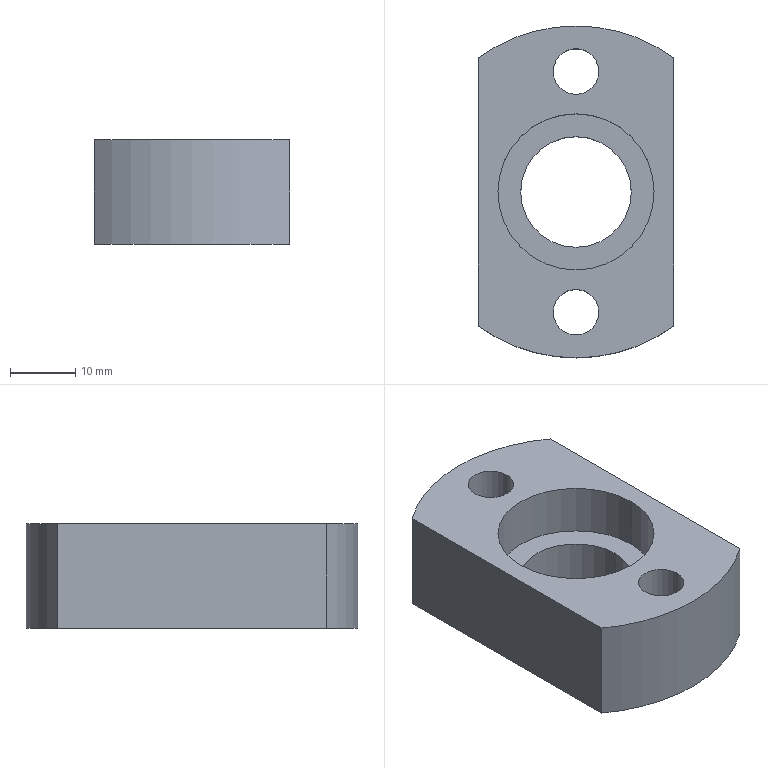Part | STEP file | qnSceondFJMC8part4 | 1 solid | 21 faces | box 30 x 51 x 16 mm | volume 15639 mm3 | cylinder 14 | plane 7 | commonest cylinder face diameters 7 x4 11 x4 17 x2 24 x2 51 x2
STEP:
#1=CARTESIAN_POINT('',(0.,0.,0.));
#2=DIRECTION('',(0.,0.,1.));
#3=DIRECTION('',(1.,0.,0.));
#4=AXIS2_PLACEMENT_3D('',#1,#2,#3);
#5=CARTESIAN_POINT('',(5.5,-18.5,0.));
#6=VERTEX_POINT('',#5);
#7=CARTESIAN_POINT('',(5.5,-18.5,6.));
#8=VERTEX_POINT('',#7);
#9=CARTESIAN_POINT('',(5.5,-18.5,0.));
#10=DIRECTION('',(0.,0.,1.));
#11=VECTOR('',#10,1.);
#12=LINE('',#9,#11);
#13=CARTESIAN_POINT('',(0.,-18.5,0.));
#14=DIRECTION('',(0.,0.,1.));
#15=DIRECTION('',(1.,0.,0.));
#16=AXIS2_PLACEMENT_3D('',#13,#14,#15);
#17=CYLINDRICAL_SURFACE('',#16,5.5);
#18=CARTESIAN_POINT('',(6.283,0.));
#19=DIRECTION('',(0.,1.));
#20=VECTOR('',#19,1.);
#21=LINE('',#18,#20);
#22=(GEOMETRIC_REPRESENTATION_CONTEXT(2)PARAMETRIC_REPRESENTATION_CONTEXT()REPRESENTATION_CONTEXT('',''));
#23=DEFINITIONAL_REPRESENTATION('',(#21),#22);
#24=PCURVE('',#17,#23);
#25=CARTESIAN_POINT('',(0.,-18.5,0.));
#26=DIRECTION('',(0.,0.,1.));
#27=DIRECTION('',(1.,0.,0.));
#28=AXIS2_PLACEMENT_3D('',#25,#26,#27);
#29=CYLINDRICAL_SURFACE('',#28,5.5);
#30=CARTESIAN_POINT('',(0.,0.));
#31=DIRECTION('',(0.,1.));
#32=VECTOR('',#31,1.);
#33=LINE('',#30,#32);
#34=(GEOMETRIC_REPRESENTATION_CONTEXT(2)PARAMETRIC_REPRESENTATION_CONTEXT()REPRESENTATION_CONTEXT('',''));
#35=DEFINITIONAL_REPRESENTATION('',(#33),#34);
#36=PCURVE('',#29,#35);
#37=SURFACE_CURVE('',#12,(#24,#36),.PCURVE_S1.);
#38=EDGE_CURVE('',#6,#8,#37,.T.);
#39=ORIENTED_EDGE('',*,*,#38,.T.);
#40=CARTESIAN_POINT('',(-5.5,-18.5,6.));
#41=VERTEX_POINT('',#40);
#42=CARTESIAN_POINT('',(0.,-18.5,6.));
#43=DIRECTION('',(0.,0.,1.));
#44=DIRECTION('',(1.,0.,0.));
#45=AXIS2_PLACEMENT_3D('',#42,#43,#44);
#46=CIRCLE('',#45,5.5);
#47=CARTESIAN_POINT('',(0.,6.));
#48=DIRECTION('',(1.,0.));
#49=VECTOR('',#48,1.);
#50=LINE('',#47,#49);
#51=(GEOMETRIC_REPRESENTATION_CONTEXT(2)PARAMETRIC_REPRESENTATION_CONTEXT()REPRESENTATION_CONTEXT('',''));
#52=DEFINITIONAL_REPRESENTATION('',(#50),#51);
#53=PCURVE('',#17,#52);
#54=CARTESIAN_POINT('',(0.,-15.,6.));
#55=DIRECTION('',(0.,0.,-1.));
#56=DIRECTION('',(-1.,0.,0.));
#57=AXIS2_PLACEMENT_3D('',#54,#55,#56);
#58=PLANE('',#57);
#59=CARTESIAN_POINT('',(-5.5,-3.5));
#60=CARTESIAN_POINT('',(-5.5,6.026));
#61=CARTESIAN_POINT('',(2.75,1.263));
#62=CARTESIAN_POINT('',(11.,-3.5));
#63=CARTESIAN_POINT('',(2.75,-8.263));
#64=CARTESIAN_POINT('',(-5.5,-13.026));
#65=CARTESIAN_POINT('',(-5.5,-3.5));
#66=(BOUNDED_CURVE()B_SPLINE_CURVE(2,(#59,#60,#61,#62,#63,#64,#65),.UNSPECIFIED.,.T.,.F.)B_SPLINE_CURVE_WITH_KNOTS((1,2,2,2,2,1),(-2.094,0.,2.094,4.189,6.283,8.378),.UNSPECIFIED.)CURVE()GEOMETRIC_REPRESENTATION_ITEM()RATIONAL_B_SPLINE_CURVE((1.,0.5,1.,0.5,1.,0.5,1.))REPRESENTATION_ITEM(''));
#67=(GEOMETRIC_REPRESENTATION_CONTEXT(2)PARAMETRIC_REPRESENTATION_CONTEXT()REPRESENTATION_CONTEXT('',''));
#68=DEFINITIONAL_REPRESENTATION('',(#66),#67);
#69=PCURVE('',#58,#68);
#70=SURFACE_CURVE('',#46,(#53,#69),.PCURVE_S1.);
#71=EDGE_CURVE('',#41,#8,#70,.T.);
#72=ORIENTED_EDGE('',*,*,#71,.F.);
#73=CARTESIAN_POINT('',(-5.5,-18.5,0.));
#74=VERTEX_POINT('',#73);
#75=CARTESIAN_POINT('',(-5.5,-18.5,0.));
#76=DIRECTION('',(0.,0.,1.));
#77=VECTOR('',#76,1.);
#78=LINE('',#75,#77);
#79=CARTESIAN_POINT('',(3.142,0.));
#80=DIRECTION('',(0.,1.));
#81=VECTOR('',#80,1.);
#82=LINE('',#79,#81);
#83=(GEOMETRIC_REPRESENTATION_CONTEXT(2)PARAMETRIC_REPRESENTATION_CONTEXT()REPRESENTATION_CONTEXT('',''));
#84=DEFINITIONAL_REPRESENTATION('',(#82),#83);
#85=PCURVE('',#17,#84);
#86=CARTESIAN_POINT('',(3.142,0.));
#87=DIRECTION('',(0.,1.));
#88=VECTOR('',#87,1.);
#89=LINE('',#86,#88);
#90=(GEOMETRIC_REPRESENTATION_CONTEXT(2)PARAMETRIC_REPRESENTATION_CONTEXT()REPRESENTATION_CONTEXT('',''));
#91=DEFINITIONAL_REPRESENTATION('',(#89),#90);
#92=PCURVE('',#29,#91);
#93=SURFACE_CURVE('',#78,(#85,#92),.PCURVE_S1.);
#94=EDGE_CURVE('',#74,#41,#93,.T.);
#95=ORIENTED_EDGE('',*,*,#94,.F.);
#96=CARTESIAN_POINT('',(0.,-18.5,0.));
#97=DIRECTION('',(0.,0.,1.));
#98=DIRECTION('',(1.,0.,0.));
#99=AXIS2_PLACEMENT_3D('',#96,#97,#98);
#100=CIRCLE('',#99,5.5);
#101=CARTESIAN_POINT('',(0.,0.));
#102=DIRECTION('',(1.,0.));
#103=VECTOR('',#102,1.);
#104=LINE('',#101,#103);
#105=(GEOMETRIC_REPRESENTATION_CONTEXT(2)PARAMETRIC_REPRESENTATION_CONTEXT()REPRESENTATION_CONTEXT('',''));
#106=DEFINITIONAL_REPRESENTATION('',(#104),#105);
#107=PCURVE('',#17,#106);
#108=CARTESIAN_POINT('',(0.,0.,0.));
#109=DIRECTION('',(0.,0.,1.));
#110=DIRECTION('',(1.,0.,0.));
#111=AXIS2_PLACEMENT_3D('',#108,#109,#110);
#112=PLANE('',#111);
#113=CARTESIAN_POINT('',(0.,-18.5));
#114=DIRECTION('',(1.,0.));
#115=AXIS2_PLACEMENT_2D('',#113,#114);
#116=CIRCLE('',#115,5.5);
#117=(GEOMETRIC_REPRESENTATION_CONTEXT(2)PARAMETRIC_REPRESENTATION_CONTEXT()REPRESENTATION_CONTEXT('',''));
#118=DEFINITIONAL_REPRESENTATION('',(#116),#117);
#119=PCURVE('',#112,#118);
#120=SURFACE_CURVE('',#100,(#107,#119),.PCURVE_S1.);
#121=EDGE_CURVE('',#74,#6,#120,.T.);
#122=ORIENTED_EDGE('',*,*,#121,.T.);
#123=EDGE_LOOP('',(#39,#72,#95,#122));
#124=FACE_BOUND('',#123,.F.);
#125=ADVANCED_FACE('',(#124),#17,.F.);
#126=CARTESIAN_POINT('',(3.5,-18.5,6.));
#127=VERTEX_POINT('',#126);
#128=CARTESIAN_POINT('',(3.5,-18.5,16.));
#129=VERTEX_POINT('',#128);
#130=CARTESIAN_POINT('',(3.5,-18.5,0.));
#131=DIRECTION('',(0.,0.,1.));
#132=VECTOR('',#131,1.);
#133=LINE('',#130,#132);
#134=CARTESIAN_POINT('',(0.,-18.5,0.));
#135=DIRECTION('',(0.,0.,1.));
#136=DIRECTION('',(1.,0.,0.));
#137=AXIS2_PLACEMENT_3D('',#134,#135,#136);
#138=CYLINDRICAL_SURFACE('',#137,3.5);
#139=CARTESIAN_POINT('',(6.283,0.));
#140=DIRECTION('',(0.,1.));
#141=VECTOR('',#140,1.);
#142=LINE('',#139,#141);
#143=(GEOMETRIC_REPRESENTATION_CONTEXT(2)PARAMETRIC_REPRESENTATION_CONTEXT()REPRESENTATION_CONTEXT('',''));
#144=DEFINITIONAL_REPRESENTATION('',(#142),#143);
#145=PCURVE('',#138,#144);
#146=CARTESIAN_POINT('',(0.,-18.5,0.));
#147=DIRECTION('',(0.,0.,1.));
#148=DIRECTION('',(1.,0.,0.));
#149=AXIS2_PLACEMENT_3D('',#146,#147,#148);
#150=CYLINDRICAL_SURFACE('',#149,3.5);
#151=CARTESIAN_POINT('',(0.,0.));
#152=DIRECTION('',(0.,1.));
#153=VECTOR('',#152,1.);
#154=LINE('',#151,#153);
#155=(GEOMETRIC_REPRESENTATION_CONTEXT(2)PARAMETRIC_REPRESENTATION_CONTEXT()REPRESENTATION_CONTEXT('',''));
#156=DEFINITIONAL_REPRESENTATION('',(#154),#155);
#157=PCURVE('',#150,#156);
#158=SURFACE_CURVE('',#133,(#145,#157),.PCURVE_S1.);
#159=EDGE_CURVE('',#127,#129,#158,.T.);
#160=ORIENTED_EDGE('',*,*,#159,.T.);
#161=CARTESIAN_POINT('',(-3.5,-18.5,16.));
#162=VERTEX_POINT('',#161);
#163=CARTESIAN_POINT('',(0.,-18.5,16.));
#164=DIRECTION('',(0.,0.,1.));
#165=DIRECTION('',(1.,0.,0.));
#166=AXIS2_PLACEMENT_3D('',#163,#164,#165);
#167=CIRCLE('',#166,3.5);
#168=CARTESIAN_POINT('',(0.,16.));
#169=DIRECTION('',(1.,0.));
#170=VECTOR('',#169,1.);
#171=LINE('',#168,#170);
#172=(GEOMETRIC_REPRESENTATION_CONTEXT(2)PARAMETRIC_REPRESENTATION_CONTEXT()REPRESENTATION_CONTEXT('',''));
#173=DEFINITIONAL_REPRESENTATION('',(#171),#172);
#174=PCURVE('',#138,#173);
#175=CARTESIAN_POINT('',(0.,0.,16.));
#176=DIRECTION('',(0.,0.,1.));
#177=DIRECTION('',(1.,0.,0.));
#178=AXIS2_PLACEMENT_3D('',#175,#176,#177);
#179=PLANE('',#178);
#180=CARTESIAN_POINT('',(0.,-18.5));
#181=DIRECTION('',(1.,0.));
#182=AXIS2_PLACEMENT_2D('',#180,#181);
#183=CIRCLE('',#182,3.5);
#184=(GEOMETRIC_REPRESENTATION_CONTEXT(2)PARAMETRIC_REPRESENTATION_CONTEXT()REPRESENTATION_CONTEXT('',''));
#185=DEFINITIONAL_REPRESENTATION('',(#183),#184);
#186=PCURVE('',#179,#185);
#187=SURFACE_CURVE('',#167,(#174,#186),.PCURVE_S1.);
#188=EDGE_CURVE('',#162,#129,#187,.T.);
#189=ORIENTED_EDGE('',*,*,#188,.F.);
#190=CARTESIAN_POINT('',(-3.5,-18.5,6.));
#191=VERTEX_POINT('',#190);
#192=CARTESIAN_POINT('',(-3.5,-18.5,0.));
#193=DIRECTION('',(0.,0.,1.));
#194=VECTOR('',#193,1.);
#195=LINE('',#192,#194);
#196=CARTESIAN_POINT('',(3.142,0.));
#197=DIRECTION('',(0.,1.));
#198=VECTOR('',#197,1.);
#199=LINE('',#196,#198);
#200=(GEOMETRIC_REPRESENTATION_CONTEXT(2)PARAMETRIC_REPRESENTATION_CONTEXT()REPRESENTATION_CONTEXT('',''));
#201=DEFINITIONAL_REPRESENTATION('',(#199),#200);
#202=PCURVE('',#138,#201);
#203=CARTESIAN_POINT('',(3.142,0.));
#204=DIRECTION('',(0.,1.));
#205=VECTOR('',#204,1.);
#206=LINE('',#203,#205);
#207=(GEOMETRIC_REPRESENTATION_CONTEXT(2)PARAMETRIC_REPRESENTATION_CONTEXT()REPRESENTATION_CONTEXT('',''));
#208=DEFINITIONAL_REPRESENTATION('',(#206),#207);
#209=PCURVE('',#150,#208);
#210=SURFACE_CURVE('',#195,(#202,#209),.PCURVE_S1.);
#211=EDGE_CURVE('',#191,#162,#210,.T.);
#212=ORIENTED_EDGE('',*,*,#211,.F.);
#213=CARTESIAN_POINT('',(0.,-18.5,6.));
#214=DIRECTION('',(0.,0.,1.));
#215=DIRECTION('',(1.,0.,0.));
#216=AXIS2_PLACEMENT_3D('',#213,#214,#215);
#217=CIRCLE('',#216,3.5);
#218=CARTESIAN_POINT('',(0.,6.));
#219=DIRECTION('',(1.,0.));
#220=VECTOR('',#219,1.);
#221=LINE('',#218,#220);
#222=(GEOMETRIC_REPRESENTATION_CONTEXT(2)PARAMETRIC_REPRESENTATION_CONTEXT()REPRESENTATION_CONTEXT('',''));
#223=DEFINITIONAL_REPRESENTATION('',(#221),#222);
#224=PCURVE('',#138,#223);
#225=CARTESIAN_POINT('',(-3.5,-3.5));
#226=CARTESIAN_POINT('',(-3.5,2.562));
#227=CARTESIAN_POINT('',(1.75,-0.4689));
#228=CARTESIAN_POINT('',(7.,-3.5));
#229=CARTESIAN_POINT('',(1.75,-6.531));
#230=CARTESIAN_POINT('',(-3.5,-9.562));
#231=CARTESIAN_POINT('',(-3.5,-3.5));
#232=(BOUNDED_CURVE()B_SPLINE_CURVE(2,(#225,#226,#227,#228,#229,#230,#231),.UNSPECIFIED.,.T.,.F.)B_SPLINE_CURVE_WITH_KNOTS((1,2,2,2,2,1),(-2.094,0.,2.094,4.189,6.283,8.378),.UNSPECIFIED.)CURVE()GEOMETRIC_REPRESENTATION_ITEM()RATIONAL_B_SPLINE_CURVE((1.,0.5,1.,0.5,1.,0.5,1.))REPRESENTATION_ITEM(''));
#233=(GEOMETRIC_REPRESENTATION_CONTEXT(2)PARAMETRIC_REPRESENTATION_CONTEXT()REPRESENTATION_CONTEXT('',''));
#234=DEFINITIONAL_REPRESENTATION('',(#232),#233);
#235=PCURVE('',#58,#234);
#236=SURFACE_CURVE('',#217,(#224,#235),.PCURVE_S1.);
#237=EDGE_CURVE('',#191,#127,#236,.T.);
#238=ORIENTED_EDGE('',*,*,#237,.T.);
#239=EDGE_LOOP('',(#160,#189,#212,#238));
#240=FACE_BOUND('',#239,.F.);
#241=ADVANCED_FACE('',(#240),#138,.F.);
#242=CARTESIAN_POINT('',(5.5,18.5,0.));
#243=VERTEX_POINT('',#242);
#244=CARTESIAN_POINT('',(5.5,18.5,6.));
#245=VERTEX_POINT('',#244);
#246=CARTESIAN_POINT('',(5.5,18.5,0.));
#247=DIRECTION('',(0.,0.,1.));
#248=VECTOR('',#247,1.);
#249=LINE('',#246,#248);
#250=CARTESIAN_POINT('',(0.,18.5,0.));
#251=DIRECTION('',(0.,0.,1.));
#252=DIRECTION('',(1.,0.,0.));
#253=AXIS2_PLACEMENT_3D('',#250,#251,#252);
#254=CYLINDRICAL_SURFACE('',#253,5.5);
#255=CARTESIAN_POINT('',(6.283,0.));
#256=DIRECTION('',(0.,1.));
#257=VECTOR('',#256,1.);
#258=LINE('',#255,#257);
#259=(GEOMETRIC_REPRESENTATION_CONTEXT(2)PARAMETRIC_REPRESENTATION_CONTEXT()REPRESENTATION_CONTEXT('',''));
#260=DEFINITIONAL_REPRESENTATION('',(#258),#259);
#261=PCURVE('',#254,#260);
#262=CARTESIAN_POINT('',(0.,18.5,0.));
#263=DIRECTION('',(0.,0.,1.));
#264=DIRECTION('',(1.,0.,0.));
#265=AXIS2_PLACEMENT_3D('',#262,#263,#264);
#266=CYLINDRICAL_SURFACE('',#265,5.5);
#267=CARTESIAN_POINT('',(0.,0.));
#268=DIRECTION('',(0.,1.));
#269=VECTOR('',#268,1.);
#270=LINE('',#267,#269);
#271=(GEOMETRIC_REPRESENTATION_CONTEXT(2)PARAMETRIC_REPRESENTATION_CONTEXT()REPRESENTATION_CONTEXT('',''));
#272=DEFINITIONAL_REPRESENTATION('',(#270),#271);
#273=PCURVE('',#266,#272);
#274=SURFACE_CURVE('',#249,(#261,#273),.PCURVE_S1.);
#275=EDGE_CURVE('',#243,#245,#274,.T.);
#276=ORIENTED_EDGE('',*,*,#275,.T.);
#277=CARTESIAN_POINT('',(-5.5,18.5,6.));
#278=VERTEX_POINT('',#277);
#279=CARTESIAN_POINT('',(0.,18.5,6.));
#280=DIRECTION('',(0.,0.,1.));
#281=DIRECTION('',(1.,0.,0.));
#282=AXIS2_PLACEMENT_3D('',#279,#280,#281);
#283=CIRCLE('',#282,5.5);
#284=CARTESIAN_POINT('',(0.,6.));
#285=DIRECTION('',(1.,0.));
#286=VECTOR('',#285,1.);
#287=LINE('',#284,#286);
#288=(GEOMETRIC_REPRESENTATION_CONTEXT(2)PARAMETRIC_REPRESENTATION_CONTEXT()REPRESENTATION_CONTEXT('',''));
#289=DEFINITIONAL_REPRESENTATION('',(#287),#288);
#290=PCURVE('',#254,#289);
#291=CARTESIAN_POINT('',(0.,22.,6.));
#292=DIRECTION('',(0.,0.,-1.));
#293=DIRECTION('',(-1.,0.,0.));
#294=AXIS2_PLACEMENT_3D('',#291,#292,#293);
#295=PLANE('',#294);
#296=CARTESIAN_POINT('',(-5.5,-3.5));
#297=CARTESIAN_POINT('',(-5.5,6.026));
#298=CARTESIAN_POINT('',(2.75,1.263));
#299=CARTESIAN_POINT('',(11.,-3.5));
#300=CARTESIAN_POINT('',(2.75,-8.263));
#301=CARTESIAN_POINT('',(-5.5,-13.026));
#302=CARTESIAN_POINT('',(-5.5,-3.5));
#303=(BOUNDED_CURVE()B_SPLINE_CURVE(2,(#296,#297,#298,#299,#300,#301,#302),.UNSPECIFIED.,.T.,.F.)B_SPLINE_CURVE_WITH_KNOTS((1,2,2,2,2,1),(-2.094,0.,2.094,4.189,6.283,8.378),.UNSPECIFIED.)CURVE()GEOMETRIC_REPRESENTATION_ITEM()RATIONAL_B_SPLINE_CURVE((1.,0.5,1.,0.5,1.,0.5,1.))REPRESENTATION_ITEM(''));
#304=(GEOMETRIC_REPRESENTATION_CONTEXT(2)PARAMETRIC_REPRESENTATION_CONTEXT()REPRESENTATION_CONTEXT('',''));
#305=DEFINITIONAL_REPRESENTATION('',(#303),#304);
#306=PCURVE('',#295,#305);
#307=SURFACE_CURVE('',#283,(#290,#306),.PCURVE_S1.);
#308=EDGE_CURVE('',#278,#245,#307,.T.);
#309=ORIENTED_EDGE('',*,*,#308,.F.);
#310=CARTESIAN_POINT('',(-5.5,18.5,0.));
#311=VERTEX_POINT('',#310);
#312=CARTESIAN_POINT('',(-5.5,18.5,0.));
#313=DIRECTION('',(0.,0.,1.));
#314=VECTOR('',#313,1.);
#315=LINE('',#312,#314);
#316=CARTESIAN_POINT('',(3.142,0.));
#317=DIRECTION('',(0.,1.));
#318=VECTOR('',#317,1.);
#319=LINE('',#316,#318);
#320=(GEOMETRIC_REPRESENTATION_CONTEXT(2)PARAMETRIC_REPRESENTATION_CONTEXT()REPRESENTATION_CONTEXT('',''));
#321=DEFINITIONAL_REPRESENTATION('',(#319),#320);
#322=PCURVE('',#254,#321);
#323=CARTESIAN_POINT('',(3.142,0.));
#324=DIRECTION('',(0.,1.));
#325=VECTOR('',#324,1.);
#326=LINE('',#323,#325);
#327=(GEOMETRIC_REPRESENTATION_CONTEXT(2)PARAMETRIC_REPRESENTATION_CONTEXT()REPRESENTATION_CONTEXT('',''));
#328=DEFINITIONAL_REPRESENTATION('',(#326),#327);
#329=PCURVE('',#266,#328);
#330=SURFACE_CURVE('',#315,(#322,#329),.PCURVE_S1.);
#331=EDGE_CURVE('',#311,#278,#330,.T.);
#332=ORIENTED_EDGE('',*,*,#331,.F.);
#333=CARTESIAN_POINT('',(0.,18.5,0.));
#334=DIRECTION('',(0.,0.,1.));
#335=DIRECTION('',(1.,0.,0.));
#336=AXIS2_PLACEMENT_3D('',#333,#334,#335);
#337=CIRCLE('',#336,5.5);
#338=CARTESIAN_POINT('',(0.,0.));
#339=DIRECTION('',(1.,0.));
#340=VECTOR('',#339,1.);
#341=LINE('',#338,#340);
#342=(GEOMETRIC_REPRESENTATION_CONTEXT(2)PARAMETRIC_REPRESENTATION_CONTEXT()REPRESENTATION_CONTEXT('',''));
#343=DEFINITIONAL_REPRESENTATION('',(#341),#342);
#344=PCURVE('',#254,#343);
#345=CARTESIAN_POINT('',(0.,18.5));
#346=DIRECTION('',(1.,0.));
#347=AXIS2_PLACEMENT_2D('',#345,#346);
#348=CIRCLE('',#347,5.5);
#349=(GEOMETRIC_REPRESENTATION_CONTEXT(2)PARAMETRIC_REPRESENTATION_CONTEXT()REPRESENTATION_CONTEXT('',''));
#350=DEFINITIONAL_REPRESENTATION('',(#348),#349);
#351=PCURVE('',#112,#350);
#352=SURFACE_CURVE('',#337,(#344,#351),.PCURVE_S1.);
#353=EDGE_CURVE('',#311,#243,#352,.T.);
#354=ORIENTED_EDGE('',*,*,#353,.T.);
#355=EDGE_LOOP('',(#276,#309,#332,#354));
#356=FACE_BOUND('',#355,.F.);
#357=ADVANCED_FACE('',(#356),#254,.F.);
#358=CARTESIAN_POINT('',(3.5,18.5,6.));
#359=VERTEX_POINT('',#358);
#360=CARTESIAN_POINT('',(3.5,18.5,16.));
#361=VERTEX_POINT('',#360);
#362=CARTESIAN_POINT('',(3.5,18.5,0.));
#363=DIRECTION('',(0.,0.,1.));
#364=VECTOR('',#363,1.);
#365=LINE('',#362,#364);
#366=CARTESIAN_POINT('',(0.,18.5,0.));
#367=DIRECTION('',(0.,0.,1.));
#368=DIRECTION('',(1.,0.,0.));
#369=AXIS2_PLACEMENT_3D('',#366,#367,#368);
#370=CYLINDRICAL_SURFACE('',#369,3.5);
#371=CARTESIAN_POINT('',(6.283,0.));
#372=DIRECTION('',(0.,1.));
#373=VECTOR('',#372,1.);
#374=LINE('',#371,#373);
#375=(GEOMETRIC_REPRESENTATION_CONTEXT(2)PARAMETRIC_REPRESENTATION_CONTEXT()REPRESENTATION_CONTEXT('',''));
#376=DEFINITIONAL_REPRESENTATION('',(#374),#375);
#377=PCURVE('',#370,#376);
#378=CARTESIAN_POINT('',(0.,18.5,0.));
#379=DIRECTION('',(0.,0.,1.));
#380=DIRECTION('',(1.,0.,0.));
#381=AXIS2_PLACEMENT_3D('',#378,#379,#380);
#382=CYLINDRICAL_SURFACE('',#381,3.5);
#383=CARTESIAN_POINT('',(0.,0.));
#384=DIRECTION('',(0.,1.));
#385=VECTOR('',#384,1.);
#386=LINE('',#383,#385);
#387=(GEOMETRIC_REPRESENTATION_CONTEXT(2)PARAMETRIC_REPRESENTATION_CONTEXT()REPRESENTATION_CONTEXT('',''));
#388=DEFINITIONAL_REPRESENTATION('',(#386),#387);
#389=PCURVE('',#382,#388);
#390=SURFACE_CURVE('',#365,(#377,#389),.PCURVE_S1.);
#391=EDGE_CURVE('',#359,#361,#390,.T.);
#392=ORIENTED_EDGE('',*,*,#391,.T.);
#393=CARTESIAN_POINT('',(-3.5,18.5,16.));
#394=VERTEX_POINT('',#393);
#395=CARTESIAN_POINT('',(0.,18.5,16.));
#396=DIRECTION('',(0.,0.,1.));
#397=DIRECTION('',(1.,0.,0.));
#398=AXIS2_PLACEMENT_3D('',#395,#396,#397);
#399=CIRCLE('',#398,3.5);
#400=CARTESIAN_POINT('',(0.,16.));
#401=DIRECTION('',(1.,0.));
#402=VECTOR('',#401,1.);
#403=LINE('',#400,#402);
#404=(GEOMETRIC_REPRESENTATION_CONTEXT(2)PARAMETRIC_REPRESENTATION_CONTEXT()REPRESENTATION_CONTEXT('',''));
#405=DEFINITIONAL_REPRESENTATION('',(#403),#404);
#406=PCURVE('',#370,#405);
#407=CARTESIAN_POINT('',(0.,18.5));
#408=DIRECTION('',(1.,0.));
#409=AXIS2_PLACEMENT_2D('',#407,#408);
#410=CIRCLE('',#409,3.5);
#411=(GEOMETRIC_REPRESENTATION_CONTEXT(2)PARAMETRIC_REPRESENTATION_CONTEXT()REPRESENTATION_CONTEXT('',''));
#412=DEFINITIONAL_REPRESENTATION('',(#410),#411);
#413=PCURVE('',#179,#412);
#414=SURFACE_CURVE('',#399,(#406,#413),.PCURVE_S1.);
#415=EDGE_CURVE('',#394,#361,#414,.T.);
#416=ORIENTED_EDGE('',*,*,#415,.F.);
#417=CARTESIAN_POINT('',(-3.5,18.5,6.));
#418=VERTEX_POINT('',#417);
#419=CARTESIAN_POINT('',(-3.5,18.5,0.));
#420=DIRECTION('',(0.,0.,1.));
#421=VECTOR('',#420,1.);
#422=LINE('',#419,#421);
#423=CARTESIAN_POINT('',(3.142,0.));
#424=DIRECTION('',(0.,1.));
#425=VECTOR('',#424,1.);
#426=LINE('',#423,#425);
#427=(GEOMETRIC_REPRESENTATION_CONTEXT(2)PARAMETRIC_REPRESENTATION_CONTEXT()REPRESENTATION_CONTEXT('',''));
#428=DEFINITIONAL_REPRESENTATION('',(#426),#427);
#429=PCURVE('',#370,#428);
#430=CARTESIAN_POINT('',(3.142,0.));
#431=DIRECTION('',(0.,1.));
#432=VECTOR('',#431,1.);
#433=LINE('',#430,#432);
#434=(GEOMETRIC_REPRESENTATION_CONTEXT(2)PARAMETRIC_REPRESENTATION_CONTEXT()REPRESENTATION_CONTEXT('',''));
#435=DEFINITIONAL_REPRESENTATION('',(#433),#434);
#436=PCURVE('',#382,#435);
#437=SURFACE_CURVE('',#422,(#429,#436),.PCURVE_S1.);
#438=EDGE_CURVE('',#418,#394,#437,.T.);
#439=ORIENTED_EDGE('',*,*,#438,.F.);
#440=CARTESIAN_POINT('',(0.,18.5,6.));
#441=DIRECTION('',(0.,0.,1.));
#442=DIRECTION('',(1.,0.,0.));
#443=AXIS2_PLACEMENT_3D('',#440,#441,#442);
#444=CIRCLE('',#443,3.5);
#445=CARTESIAN_POINT('',(0.,6.));
#446=DIRECTION('',(1.,0.));
#447=VECTOR('',#446,1.);
#448=LINE('',#445,#447);
#449=(GEOMETRIC_REPRESENTATION_CONTEXT(2)PARAMETRIC_REPRESENTATION_CONTEXT()REPRESENTATION_CONTEXT('',''));
#450=DEFINITIONAL_REPRESENTATION('',(#448),#449);
#451=PCURVE('',#370,#450);
#452=CARTESIAN_POINT('',(-3.5,-3.5));
#453=CARTESIAN_POINT('',(-3.5,2.562));
#454=CARTESIAN_POINT('',(1.75,-0.4689));
#455=CARTESIAN_POINT('',(7.,-3.5));
#456=CARTESIAN_POINT('',(1.75,-6.531));
#457=CARTESIAN_POINT('',(-3.5,-9.562));
#458=CARTESIAN_POINT('',(-3.5,-3.5));
#459=(BOUNDED_CURVE()B_SPLINE_CURVE(2,(#452,#453,#454,#455,#456,#457,#458),.UNSPECIFIED.,.T.,.F.)B_SPLINE_CURVE_WITH_KNOTS((1,2,2,2,2,1),(-2.094,0.,2.094,4.189,6.283,8.378),.UNSPECIFIED.)CURVE()GEOMETRIC_REPRESENTATION_ITEM()RATIONAL_B_SPLINE_CURVE((1.,0.5,1.,0.5,1.,0.5,1.))REPRESENTATION_ITEM(''));
#460=(GEOMETRIC_REPRESENTATION_CONTEXT(2)PARAMETRIC_REPRESENTATION_CONTEXT()REPRESENTATION_CONTEXT('',''));
#461=DEFINITIONAL_REPRESENTATION('',(#459),#460);
#462=PCURVE('',#295,#461);
#463=SURFACE_CURVE('',#444,(#451,#462),.PCURVE_S1.);
#464=EDGE_CURVE('',#418,#359,#463,.T.);
#465=ORIENTED_EDGE('',*,*,#464,.T.);
#466=EDGE_LOOP('',(#392,#416,#439,#465));
#467=FACE_BOUND('',#466,.F.);
#468=ADVANCED_FACE('',(#467),#370,.F.);
#469=CARTESIAN_POINT('',(8.5,0.,0.));
#470=VERTEX_POINT('',#469);
#471=CARTESIAN_POINT('',(8.5,0.,8.));
#472=VERTEX_POINT('',#471);
#473=CARTESIAN_POINT('',(8.5,0.,0.));
#474=DIRECTION('',(0.,0.,1.));
#475=VECTOR('',#474,1.);
#476=LINE('',#473,#475);
#477=CARTESIAN_POINT('',(0.,0.,0.));
#478=DIRECTION('',(0.,0.,1.));
#479=DIRECTION('',(1.,0.,0.));
#480=AXIS2_PLACEMENT_3D('',#477,#478,#479);
#481=CYLINDRICAL_SURFACE('',#480,8.5);
#482=CARTESIAN_POINT('',(6.283,0.));
#483=DIRECTION('',(0.,1.));
#484=VECTOR('',#483,1.);
#485=LINE('',#482,#484);
#486=(GEOMETRIC_REPRESENTATION_CONTEXT(2)PARAMETRIC_REPRESENTATION_CONTEXT()REPRESENTATION_CONTEXT('',''));
#487=DEFINITIONAL_REPRESENTATION('',(#485),#486);
#488=PCURVE('',#481,#487);
#489=CARTESIAN_POINT('',(0.,0.,0.));
#490=DIRECTION('',(0.,0.,1.));
#491=DIRECTION('',(1.,0.,0.));
#492=AXIS2_PLACEMENT_3D('',#489,#490,#491);
#493=CYLINDRICAL_SURFACE('',#492,8.5);
#494=CARTESIAN_POINT('',(0.,0.));
#495=DIRECTION('',(0.,1.));
#496=VECTOR('',#495,1.);
#497=LINE('',#494,#496);
#498=(GEOMETRIC_REPRESENTATION_CONTEXT(2)PARAMETRIC_REPRESENTATION_CONTEXT()REPRESENTATION_CONTEXT('',''));
#499=DEFINITIONAL_REPRESENTATION('',(#497),#498);
#500=PCURVE('',#493,#499);
#501=SURFACE_CURVE('',#476,(#488,#500),.PCURVE_S1.);
#502=EDGE_CURVE('',#470,#472,#501,.T.);
#503=ORIENTED_EDGE('',*,*,#502,.T.);
#504=CARTESIAN_POINT('',(-8.5,0.,8.));
#505=VERTEX_POINT('',#504);
#506=CARTESIAN_POINT('',(0.,0.,8.));
#507=DIRECTION('',(0.,0.,1.));
#508=DIRECTION('',(1.,0.,0.));
#509=AXIS2_PLACEMENT_3D('',#506,#507,#508);
#510=CIRCLE('',#509,8.5);
#511=CARTESIAN_POINT('',(0.,8.));
#512=DIRECTION('',(1.,0.));
#513=VECTOR('',#512,1.);
#514=LINE('',#511,#513);
#515=(GEOMETRIC_REPRESENTATION_CONTEXT(2)PARAMETRIC_REPRESENTATION_CONTEXT()REPRESENTATION_CONTEXT('',''));
#516=DEFINITIONAL_REPRESENTATION('',(#514),#515);
#517=PCURVE('',#481,#516);
#518=CARTESIAN_POINT('',(0.,12.,8.));
#519=DIRECTION('',(0.,0.,1.));
#520=DIRECTION('',(1.,0.,0.));
#521=AXIS2_PLACEMENT_3D('',#518,#519,#520);
#522=PLANE('',#521);
#523=CARTESIAN_POINT('',(0.,-12.));
#524=DIRECTION('',(1.,0.));
#525=AXIS2_PLACEMENT_2D('',#523,#524);
#526=CIRCLE('',#525,8.5);
#527=(GEOMETRIC_REPRESENTATION_CONTEXT(2)PARAMETRIC_REPRESENTATION_CONTEXT()REPRESENTATION_CONTEXT('',''));
#528=DEFINITIONAL_REPRESENTATION('',(#526),#527);
#529=PCURVE('',#522,#528);
#530=SURFACE_CURVE('',#510,(#517,#529),.PCURVE_S1.);
#531=EDGE_CURVE('',#505,#472,#530,.T.);
#532=ORIENTED_EDGE('',*,*,#531,.F.);
#533=CARTESIAN_POINT('',(-8.5,0.,0.));
#534=VERTEX_POINT('',#533);
#535=CARTESIAN_POINT('',(-8.5,0.,0.));
#536=DIRECTION('',(0.,0.,1.));
#537=VECTOR('',#536,1.);
#538=LINE('',#535,#537);
#539=CARTESIAN_POINT('',(3.142,0.));
#540=DIRECTION('',(0.,1.));
#541=VECTOR('',#540,1.);
#542=LINE('',#539,#541);
#543=(GEOMETRIC_REPRESENTATION_CONTEXT(2)PARAMETRIC_REPRESENTATION_CONTEXT()REPRESENTATION_CONTEXT('',''));
#544=DEFINITIONAL_REPRESENTATION('',(#542),#543);
#545=PCURVE('',#481,#544);
#546=CARTESIAN_POINT('',(3.142,0.));
#547=DIRECTION('',(0.,1.));
#548=VECTOR('',#547,1.);
#549=LINE('',#546,#548);
#550=(GEOMETRIC_REPRESENTATION_CONTEXT(2)PARAMETRIC_REPRESENTATION_CONTEXT()REPRESENTATION_CONTEXT('',''));
#551=DEFINITIONAL_REPRESENTATION('',(#549),#550);
#552=PCURVE('',#493,#551);
#553=SURFACE_CURVE('',#538,(#545,#552),.PCURVE_S1.);
#554=EDGE_CURVE('',#534,#505,#553,.T.);
#555=ORIENTED_EDGE('',*,*,#554,.F.);
#556=CARTESIAN_POINT('',(0.,0.,0.));
#557=DIRECTION('',(0.,0.,1.));
#558=DIRECTION('',(1.,0.,0.));
#559=AXIS2_PLACEMENT_3D('',#556,#557,#558);
#560=CIRCLE('',#559,8.5);
#561=CARTESIAN_POINT('',(0.,0.));
#562=DIRECTION('',(1.,0.));
#563=VECTOR('',#562,1.);
#564=LINE('',#561,#563);
#565=(GEOMETRIC_REPRESENTATION_CONTEXT(2)PARAMETRIC_REPRESENTATION_CONTEXT()REPRESENTATION_CONTEXT('',''));
#566=DEFINITIONAL_REPRESENTATION('',(#564),#565);
#567=PCURVE('',#481,#566);
#568=CARTESIAN_POINT('',(0.,0.));
#569=DIRECTION('',(1.,0.));
#570=AXIS2_PLACEMENT_2D('',#568,#569);
#571=CIRCLE('',#570,8.5);
#572=(GEOMETRIC_REPRESENTATION_CONTEXT(2)PARAMETRIC_REPRESENTATION_CONTEXT()REPRESENTATION_CONTEXT('',''));
#573=DEFINITIONAL_REPRESENTATION('',(#571),#572);
#574=PCURVE('',#112,#573);
#575=SURFACE_CURVE('',#560,(#567,#574),.PCURVE_S1.);
#576=EDGE_CURVE('',#534,#470,#575,.T.);
#577=ORIENTED_EDGE('',*,*,#576,.T.);
#578=EDGE_LOOP('',(#503,#532,#555,#577));
#579=FACE_BOUND('',#578,.F.);
#580=ADVANCED_FACE('',(#579),#481,.F.);
#581=CARTESIAN_POINT('',(12.,0.,8.));
#582=VERTEX_POINT('',#581);
#583=CARTESIAN_POINT('',(12.,0.,16.));
#584=VERTEX_POINT('',#583);
#585=CARTESIAN_POINT('',(12.,0.,0.));
#586=DIRECTION('',(0.,0.,1.));
#587=VECTOR('',#586,1.);
#588=LINE('',#585,#587);
#589=CARTESIAN_POINT('',(0.,0.,0.));
#590=DIRECTION('',(0.,0.,1.));
#591=DIRECTION('',(1.,0.,0.));
#592=AXIS2_PLACEMENT_3D('',#589,#590,#591);
#593=CYLINDRICAL_SURFACE('',#592,12.);
#594=CARTESIAN_POINT('',(6.283,0.));
#595=DIRECTION('',(0.,1.));
#596=VECTOR('',#595,1.);
#597=LINE('',#594,#596);
#598=(GEOMETRIC_REPRESENTATION_CONTEXT(2)PARAMETRIC_REPRESENTATION_CONTEXT()REPRESENTATION_CONTEXT('',''));
#599=DEFINITIONAL_REPRESENTATION('',(#597),#598);
#600=PCURVE('',#593,#599);
#601=CARTESIAN_POINT('',(0.,0.,0.));
#602=DIRECTION('',(0.,0.,1.));
#603=DIRECTION('',(1.,0.,0.));
#604=AXIS2_PLACEMENT_3D('',#601,#602,#603);
#605=CYLINDRICAL_SURFACE('',#604,12.);
#606=CARTESIAN_POINT('',(0.,0.));
#607=DIRECTION('',(0.,1.));
#608=VECTOR('',#607,1.);
#609=LINE('',#606,#608);
#610=(GEOMETRIC_REPRESENTATION_CONTEXT(2)PARAMETRIC_REPRESENTATION_CONTEXT()REPRESENTATION_CONTEXT('',''));
#611=DEFINITIONAL_REPRESENTATION('',(#609),#610);
#612=PCURVE('',#605,#611);
#613=SURFACE_CURVE('',#588,(#600,#612),.PCURVE_S1.);
#614=EDGE_CURVE('',#582,#584,#613,.T.);
#615=ORIENTED_EDGE('',*,*,#614,.T.);
#616=CARTESIAN_POINT('',(-12.,0.,16.));
#617=VERTEX_POINT('',#616);
#618=CARTESIAN_POINT('',(0.,0.,16.));
#619=DIRECTION('',(0.,0.,1.));
#620=DIRECTION('',(1.,0.,0.));
#621=AXIS2_PLACEMENT_3D('',#618,#619,#620);
#622=CIRCLE('',#621,12.);
#623=CARTESIAN_POINT('',(0.,16.));
#624=DIRECTION('',(1.,0.));
#625=VECTOR('',#624,1.);
#626=LINE('',#623,#625);
#627=(GEOMETRIC_REPRESENTATION_CONTEXT(2)PARAMETRIC_REPRESENTATION_CONTEXT()REPRESENTATION_CONTEXT('',''));
#628=DEFINITIONAL_REPRESENTATION('',(#626),#627);
#629=PCURVE('',#593,#628);
#630=CARTESIAN_POINT('',(0.,0.));
#631=DIRECTION('',(1.,0.));
#632=AXIS2_PLACEMENT_2D('',#630,#631);
#633=CIRCLE('',#632,12.);
#634=(GEOMETRIC_REPRESENTATION_CONTEXT(2)PARAMETRIC_REPRESENTATION_CONTEXT()REPRESENTATION_CONTEXT('',''));
#635=DEFINITIONAL_REPRESENTATION('',(#633),#634);
#636=PCURVE('',#179,#635);
#637=SURFACE_CURVE('',#622,(#629,#636),.PCURVE_S1.);
#638=EDGE_CURVE('',#617,#584,#637,.T.);
#639=ORIENTED_EDGE('',*,*,#638,.F.);
#640=CARTESIAN_POINT('',(-12.,0.,8.));
#641=VERTEX_POINT('',#640);
#642=CARTESIAN_POINT('',(-12.,0.,0.));
#643=DIRECTION('',(0.,0.,1.));
#644=VECTOR('',#643,1.);
#645=LINE('',#642,#644);
#646=CARTESIAN_POINT('',(3.142,0.));
#647=DIRECTION('',(0.,1.));
#648=VECTOR('',#647,1.);
#649=LINE('',#646,#648);
#650=(GEOMETRIC_REPRESENTATION_CONTEXT(2)PARAMETRIC_REPRESENTATION_CONTEXT()REPRESENTATION_CONTEXT('',''));
#651=DEFINITIONAL_REPRESENTATION('',(#649),#650);
#652=PCURVE('',#593,#651);
#653=CARTESIAN_POINT('',(3.142,0.));
#654=DIRECTION('',(0.,1.));
#655=VECTOR('',#654,1.);
#656=LINE('',#653,#655);
#657=(GEOMETRIC_REPRESENTATION_CONTEXT(2)PARAMETRIC_REPRESENTATION_CONTEXT()REPRESENTATION_CONTEXT('',''));
#658=DEFINITIONAL_REPRESENTATION('',(#656),#657);
#659=PCURVE('',#605,#658);
#660=SURFACE_CURVE('',#645,(#652,#659),.PCURVE_S1.);
#661=EDGE_CURVE('',#641,#617,#660,.T.);
#662=ORIENTED_EDGE('',*,*,#661,.F.);
#663=CARTESIAN_POINT('',(0.,0.,8.));
#664=DIRECTION('',(0.,0.,1.));
#665=DIRECTION('',(1.,0.,0.));
#666=AXIS2_PLACEMENT_3D('',#663,#664,#665);
#667=CIRCLE('',#666,12.);
#668=CARTESIAN_POINT('',(0.,8.));
#669=DIRECTION('',(1.,0.));
#670=VECTOR('',#669,1.);
#671=LINE('',#668,#670);
#672=(GEOMETRIC_REPRESENTATION_CONTEXT(2)PARAMETRIC_REPRESENTATION_CONTEXT()REPRESENTATION_CONTEXT('',''));
#673=DEFINITIONAL_REPRESENTATION('',(#671),#672);
#674=PCURVE('',#593,#673);
#675=CARTESIAN_POINT('',(0.,-12.));
#676=DIRECTION('',(1.,0.));
#677=AXIS2_PLACEMENT_2D('',#675,#676);
#678=CIRCLE('',#677,12.);
#679=(GEOMETRIC_REPRESENTATION_CONTEXT(2)PARAMETRIC_REPRESENTATION_CONTEXT()REPRESENTATION_CONTEXT('',''));
#680=DEFINITIONAL_REPRESENTATION('',(#678),#679);
#681=PCURVE('',#522,#680);
#682=SURFACE_CURVE('',#667,(#674,#681),.PCURVE_S1.);
#683=EDGE_CURVE('',#641,#582,#682,.T.);
#684=ORIENTED_EDGE('',*,*,#683,.T.);
#685=EDGE_LOOP('',(#615,#639,#662,#684));
#686=FACE_BOUND('',#685,.F.);
#687=ADVANCED_FACE('',(#686),#593,.F.);
#688=CARTESIAN_POINT('',(0.,18.5,16.));
#689=DIRECTION('',(0.,0.,1.));
#690=DIRECTION('',(1.,0.,0.));
#691=AXIS2_PLACEMENT_3D('',#688,#689,#690);
#692=CIRCLE('',#691,3.5);
#693=CARTESIAN_POINT('',(0.,18.5));
#694=DIRECTION('',(1.,0.));
#695=AXIS2_PLACEMENT_2D('',#693,#694);
#696=CIRCLE('',#695,3.5);
#697=(GEOMETRIC_REPRESENTATION_CONTEXT(2)PARAMETRIC_REPRESENTATION_CONTEXT()REPRESENTATION_CONTEXT('',''));
#698=DEFINITIONAL_REPRESENTATION('',(#696),#697);
#699=PCURVE('',#179,#698);
#700=CARTESIAN_POINT('',(0.,16.));
#701=DIRECTION('',(1.,0.));
#702=VECTOR('',#701,1.);
#703=LINE('',#700,#702);
#704=(GEOMETRIC_REPRESENTATION_CONTEXT(2)PARAMETRIC_REPRESENTATION_CONTEXT()REPRESENTATION_CONTEXT('',''));
#705=DEFINITIONAL_REPRESENTATION('',(#703),#704);
#706=PCURVE('',#382,#705);
#707=SURFACE_CURVE('',#692,(#699,#706),.PCURVE_S1.);
#708=EDGE_CURVE('',#361,#394,#707,.T.);
#709=ORIENTED_EDGE('',*,*,#708,.F.);
#710=ORIENTED_EDGE('',*,*,#415,.F.);
#711=EDGE_LOOP('',(#709,#710));
#712=FACE_BOUND('',#711,.T.);
#713=CARTESIAN_POINT('',(-15.,-20.622,16.));
#714=VERTEX_POINT('',#713);
#715=CARTESIAN_POINT('',(15.,-20.622,16.));
#716=VERTEX_POINT('',#715);
#717=CARTESIAN_POINT('',(0.,0.,16.));
#718=DIRECTION('',(0.,0.,1.));
#719=DIRECTION('',(1.,0.,0.));
#720=AXIS2_PLACEMENT_3D('',#717,#718,#719);
#721=CIRCLE('',#720,25.5);
#722=CARTESIAN_POINT('',(0.,0.));
#723=DIRECTION('',(1.,0.));
#724=AXIS2_PLACEMENT_2D('',#722,#723);
#725=CIRCLE('',#724,25.5);
#726=(GEOMETRIC_REPRESENTATION_CONTEXT(2)PARAMETRIC_REPRESENTATION_CONTEXT()REPRESENTATION_CONTEXT('',''));
#727=DEFINITIONAL_REPRESENTATION('',(#725),#726);
#728=PCURVE('',#179,#727);
#729=CARTESIAN_POINT('',(0.,0.,16.));
#730=DIRECTION('',(0.,0.,-1.));
#731=DIRECTION('',(-1.,0.,0.));
#732=AXIS2_PLACEMENT_3D('',#729,#730,#731);
#733=CYLINDRICAL_SURFACE('',#732,25.5);
#734=CARTESIAN_POINT('',(9.425,0.));
#735=DIRECTION('',(-1.,0.));
#736=VECTOR('',#735,1.);
#737=LINE('',#734,#736);
#738=(GEOMETRIC_REPRESENTATION_CONTEXT(2)PARAMETRIC_REPRESENTATION_CONTEXT()REPRESENTATION_CONTEXT('',''));
#739=DEFINITIONAL_REPRESENTATION('',(#737),#738);
#740=PCURVE('',#733,#739);
#741=SURFACE_CURVE('',#721,(#728,#740),.PCURVE_S1.);
#742=EDGE_CURVE('',#714,#716,#741,.T.);
#743=ORIENTED_EDGE('',*,*,#742,.T.);
#744=CARTESIAN_POINT('',(15.,20.622,16.));
#745=VERTEX_POINT('',#744);
#746=CARTESIAN_POINT('',(15.,-20.622,16.));
#747=DIRECTION('',(0.,1.,0.));
#748=VECTOR('',#747,1.);
#749=LINE('',#746,#748);
#750=CARTESIAN_POINT('',(15.,-20.622));
#751=DIRECTION('',(0.,1.));
#752=VECTOR('',#751,1.);
#753=LINE('',#750,#752);
#754=(GEOMETRIC_REPRESENTATION_CONTEXT(2)PARAMETRIC_REPRESENTATION_CONTEXT()REPRESENTATION_CONTEXT('',''));
#755=DEFINITIONAL_REPRESENTATION('',(#753),#754);
#756=PCURVE('',#179,#755);
#757=CARTESIAN_POINT('',(15.,-20.622,16.));
#758=DIRECTION('',(-1.,0.,0.));
#759=DIRECTION('',(0.,0.,1.));
#760=AXIS2_PLACEMENT_3D('',#757,#758,#759);
#761=PLANE('',#760);
#762=CARTESIAN_POINT('',(0.,0.));
#763=DIRECTION('',(0.,1.));
#764=VECTOR('',#763,1.);
#765=LINE('',#762,#764);
#766=(GEOMETRIC_REPRESENTATION_CONTEXT(2)PARAMETRIC_REPRESENTATION_CONTEXT()REPRESENTATION_CONTEXT('',''));
#767=DEFINITIONAL_REPRESENTATION('',(#765),#766);
#768=PCURVE('',#761,#767);
#769=SURFACE_CURVE('',#749,(#756,#768),.PCURVE_S1.);
#770=EDGE_CURVE('',#716,#745,#769,.T.);
#771=ORIENTED_EDGE('',*,*,#770,.T.);
#772=CARTESIAN_POINT('',(-15.,20.622,16.));
#773=VERTEX_POINT('',#772);
#774=CARTESIAN_POINT('',(0.,0.,16.));
#775=DIRECTION('',(0.,0.,1.));
#776=DIRECTION('',(1.,0.,0.));
#777=AXIS2_PLACEMENT_3D('',#774,#775,#776);
#778=CIRCLE('',#777,25.5);
#779=CARTESIAN_POINT('',(0.,0.));
#780=DIRECTION('',(1.,0.));
#781=AXIS2_PLACEMENT_2D('',#779,#780);
#782=CIRCLE('',#781,25.5);
#783=(GEOMETRIC_REPRESENTATION_CONTEXT(2)PARAMETRIC_REPRESENTATION_CONTEXT()REPRESENTATION_CONTEXT('',''));
#784=DEFINITIONAL_REPRESENTATION('',(#782),#783);
#785=PCURVE('',#179,#784);
#786=CARTESIAN_POINT('',(0.,0.,16.));
#787=DIRECTION('',(0.,0.,-1.));
#788=DIRECTION('',(-1.,0.,0.));
#789=AXIS2_PLACEMENT_3D('',#786,#787,#788);
#790=CYLINDRICAL_SURFACE('',#789,25.5);
#791=CARTESIAN_POINT('',(3.142,0.));
#792=DIRECTION('',(-1.,0.));
#793=VECTOR('',#792,1.);
#794=LINE('',#791,#793);
#795=(GEOMETRIC_REPRESENTATION_CONTEXT(2)PARAMETRIC_REPRESENTATION_CONTEXT()REPRESENTATION_CONTEXT('',''));
#796=DEFINITIONAL_REPRESENTATION('',(#794),#795);
#797=PCURVE('',#790,#796);
#798=SURFACE_CURVE('',#778,(#785,#797),.PCURVE_S1.);
#799=EDGE_CURVE('',#745,#773,#798,.T.);
#800=ORIENTED_EDGE('',*,*,#799,.T.);
#801=CARTESIAN_POINT('',(-15.,20.622,16.));
#802=DIRECTION('',(0.,-1.,0.));
#803=VECTOR('',#802,1.);
#804=LINE('',#801,#803);
#805=CARTESIAN_POINT('',(-15.,20.622));
#806=DIRECTION('',(0.,-1.));
#807=VECTOR('',#806,1.);
#808=LINE('',#805,#807);
#809=(GEOMETRIC_REPRESENTATION_CONTEXT(2)PARAMETRIC_REPRESENTATION_CONTEXT()REPRESENTATION_CONTEXT('',''));
#810=DEFINITIONAL_REPRESENTATION('',(#808),#809);
#811=PCURVE('',#179,#810);
#812=CARTESIAN_POINT('',(-15.,20.622,16.));
#813=DIRECTION('',(1.,0.,0.));
#814=DIRECTION('',(0.,0.,-1.));
#815=AXIS2_PLACEMENT_3D('',#812,#813,#814);
#816=PLANE('',#815);
#817=CARTESIAN_POINT('',(0.,0.));
#818=DIRECTION('',(0.,-1.));
#819=VECTOR('',#818,1.);
#820=LINE('',#817,#819);
#821=(GEOMETRIC_REPRESENTATION_CONTEXT(2)PARAMETRIC_REPRESENTATION_CONTEXT()REPRESENTATION_CONTEXT('',''));
#822=DEFINITIONAL_REPRESENTATION('',(#820),#821);
#823=PCURVE('',#816,#822);
#824=SURFACE_CURVE('',#804,(#811,#823),.PCURVE_S1.);
#825=EDGE_CURVE('',#773,#714,#824,.T.);
#826=ORIENTED_EDGE('',*,*,#825,.T.);
#827=EDGE_LOOP('',(#743,#771,#800,#826));
#828=FACE_BOUND('',#827,.T.);
#829=CARTESIAN_POINT('',(0.,0.,16.));
#830=DIRECTION('',(0.,0.,1.));
#831=DIRECTION('',(1.,0.,0.));
#832=AXIS2_PLACEMENT_3D('',#829,#830,#831);
#833=CIRCLE('',#832,12.);
#834=CARTESIAN_POINT('',(0.,0.));
#835=DIRECTION('',(1.,0.));
#836=AXIS2_PLACEMENT_2D('',#834,#835);
#837=CIRCLE('',#836,12.);
#838=(GEOMETRIC_REPRESENTATION_CONTEXT(2)PARAMETRIC_REPRESENTATION_CONTEXT()REPRESENTATION_CONTEXT('',''));
#839=DEFINITIONAL_REPRESENTATION('',(#837),#838);
#840=PCURVE('',#179,#839);
#841=CARTESIAN_POINT('',(0.,16.));
#842=DIRECTION('',(1.,0.));
#843=VECTOR('',#842,1.);
#844=LINE('',#841,#843);
#845=(GEOMETRIC_REPRESENTATION_CONTEXT(2)PARAMETRIC_REPRESENTATION_CONTEXT()REPRESENTATION_CONTEXT('',''));
#846=DEFINITIONAL_REPRESENTATION('',(#844),#845);
#847=PCURVE('',#605,#846);
#848=SURFACE_CURVE('',#833,(#840,#847),.PCURVE_S1.);
#849=EDGE_CURVE('',#584,#617,#848,.T.);
#850=ORIENTED_EDGE('',*,*,#849,.F.);
#851=ORIENTED_EDGE('',*,*,#638,.F.);
#852=EDGE_LOOP('',(#850,#851));
#853=FACE_BOUND('',#852,.T.);
#854=CARTESIAN_POINT('',(0.,-18.5,16.));
#855=DIRECTION('',(0.,0.,1.));
#856=DIRECTION('',(1.,0.,0.));
#857=AXIS2_PLACEMENT_3D('',#854,#855,#856);
#858=CIRCLE('',#857,3.5);
#859=CARTESIAN_POINT('',(0.,-18.5));
#860=DIRECTION('',(1.,0.));
#861=AXIS2_PLACEMENT_2D('',#859,#860);
#862=CIRCLE('',#861,3.5);
#863=(GEOMETRIC_REPRESENTATION_CONTEXT(2)PARAMETRIC_REPRESENTATION_CONTEXT()REPRESENTATION_CONTEXT('',''));
#864=DEFINITIONAL_REPRESENTATION('',(#862),#863);
#865=PCURVE('',#179,#864);
#866=CARTESIAN_POINT('',(0.,16.));
#867=DIRECTION('',(1.,0.));
#868=VECTOR('',#867,1.);
#869=LINE('',#866,#868);
#870=(GEOMETRIC_REPRESENTATION_CONTEXT(2)PARAMETRIC_REPRESENTATION_CONTEXT()REPRESENTATION_CONTEXT('',''));
#871=DEFINITIONAL_REPRESENTATION('',(#869),#870);
#872=PCURVE('',#150,#871);
#873=SURFACE_CURVE('',#858,(#865,#872),.PCURVE_S1.);
#874=EDGE_CURVE('',#129,#162,#873,.T.);
#875=ORIENTED_EDGE('',*,*,#874,.F.);
#876=ORIENTED_EDGE('',*,*,#188,.F.);
#877=EDGE_LOOP('',(#875,#876));
#878=FACE_BOUND('',#877,.T.);
#879=ADVANCED_FACE('',(#712,#828,#853,#878),#179,.T.);
#880=CARTESIAN_POINT('',(0.,18.5,0.));
#881=DIRECTION('',(0.,0.,1.));
#882=DIRECTION('',(1.,0.,0.));
#883=AXIS2_PLACEMENT_3D('',#880,#881,#882);
#884=CIRCLE('',#883,5.5);
#885=CARTESIAN_POINT('',(0.,18.5));
#886=DIRECTION('',(1.,0.));
#887=AXIS2_PLACEMENT_2D('',#885,#886);
#888=CIRCLE('',#887,5.5);
#889=(GEOMETRIC_REPRESENTATION_CONTEXT(2)PARAMETRIC_REPRESENTATION_CONTEXT()REPRESENTATION_CONTEXT('',''));
#890=DEFINITIONAL_REPRESENTATION('',(#888),#889);
#891=PCURVE('',#112,#890);
#892=CARTESIAN_POINT('',(0.,0.));
#893=DIRECTION('',(1.,0.));
#894=VECTOR('',#893,1.);
#895=LINE('',#892,#894);
#896=(GEOMETRIC_REPRESENTATION_CONTEXT(2)PARAMETRIC_REPRESENTATION_CONTEXT()REPRESENTATION_CONTEXT('',''));
#897=DEFINITIONAL_REPRESENTATION('',(#895),#896);
#898=PCURVE('',#266,#897);
#899=SURFACE_CURVE('',#884,(#891,#898),.PCURVE_S1.);
#900=EDGE_CURVE('',#243,#311,#899,.T.);
#901=ORIENTED_EDGE('',*,*,#900,.T.);
#902=ORIENTED_EDGE('',*,*,#353,.T.);
#903=EDGE_LOOP('',(#901,#902));
#904=FACE_BOUND('',#903,.T.);
#905=CARTESIAN_POINT('',(-15.,-20.622,0.));
#906=VERTEX_POINT('',#905);
#907=CARTESIAN_POINT('',(15.,-20.622,0.));
#908=VERTEX_POINT('',#907);
#909=CARTESIAN_POINT('',(0.,0.,0.));
#910=DIRECTION('',(0.,0.,1.));
#911=DIRECTION('',(1.,0.,0.));
#912=AXIS2_PLACEMENT_3D('',#909,#910,#911);
#913=CIRCLE('',#912,25.5);
#914=CARTESIAN_POINT('',(0.,0.));
#915=DIRECTION('',(1.,0.));
#916=AXIS2_PLACEMENT_2D('',#914,#915);
#917=CIRCLE('',#916,25.5);
#918=(GEOMETRIC_REPRESENTATION_CONTEXT(2)PARAMETRIC_REPRESENTATION_CONTEXT()REPRESENTATION_CONTEXT('',''));
#919=DEFINITIONAL_REPRESENTATION('',(#917),#918);
#920=PCURVE('',#112,#919);
#921=CARTESIAN_POINT('',(9.425,16.));
#922=DIRECTION('',(-1.,0.));
#923=VECTOR('',#922,1.);
#924=LINE('',#921,#923);
#925=(GEOMETRIC_REPRESENTATION_CONTEXT(2)PARAMETRIC_REPRESENTATION_CONTEXT()REPRESENTATION_CONTEXT('',''));
#926=DEFINITIONAL_REPRESENTATION('',(#924),#925);
#927=PCURVE('',#733,#926);
#928=SURFACE_CURVE('',#913,(#920,#927),.PCURVE_S1.);
#929=EDGE_CURVE('',#906,#908,#928,.T.);
#930=ORIENTED_EDGE('',*,*,#929,.F.);
#931=CARTESIAN_POINT('',(-15.,20.622,0.));
#932=VERTEX_POINT('',#931);
#933=CARTESIAN_POINT('',(-15.,20.622,0.));
#934=DIRECTION('',(0.,-1.,0.));
#935=VECTOR('',#934,1.);
#936=LINE('',#933,#935);
#937=CARTESIAN_POINT('',(-15.,20.622));
#938=DIRECTION('',(0.,-1.));
#939=VECTOR('',#938,1.);
#940=LINE('',#937,#939);
#941=(GEOMETRIC_REPRESENTATION_CONTEXT(2)PARAMETRIC_REPRESENTATION_CONTEXT()REPRESENTATION_CONTEXT('',''));
#942=DEFINITIONAL_REPRESENTATION('',(#940),#941);
#943=PCURVE('',#112,#942);
#944=CARTESIAN_POINT('',(16.,0.));
#945=DIRECTION('',(0.,-1.));
#946=VECTOR('',#945,1.);
#947=LINE('',#944,#946);
#948=(GEOMETRIC_REPRESENTATION_CONTEXT(2)PARAMETRIC_REPRESENTATION_CONTEXT()REPRESENTATION_CONTEXT('',''));
#949=DEFINITIONAL_REPRESENTATION('',(#947),#948);
#950=PCURVE('',#816,#949);
#951=SURFACE_CURVE('',#936,(#943,#950),.PCURVE_S1.);
#952=EDGE_CURVE('',#932,#906,#951,.T.);
#953=ORIENTED_EDGE('',*,*,#952,.F.);
#954=CARTESIAN_POINT('',(15.,20.622,0.));
#955=VERTEX_POINT('',#954);
#956=CARTESIAN_POINT('',(0.,0.,0.));
#957=DIRECTION('',(0.,0.,1.));
#958=DIRECTION('',(1.,0.,0.));
#959=AXIS2_PLACEMENT_3D('',#956,#957,#958);
#960=CIRCLE('',#959,25.5);
#961=CARTESIAN_POINT('',(0.,0.));
#962=DIRECTION('',(1.,0.));
#963=AXIS2_PLACEMENT_2D('',#961,#962);
#964=CIRCLE('',#963,25.5);
#965=(GEOMETRIC_REPRESENTATION_CONTEXT(2)PARAMETRIC_REPRESENTATION_CONTEXT()REPRESENTATION_CONTEXT('',''));
#966=DEFINITIONAL_REPRESENTATION('',(#964),#965);
#967=PCURVE('',#112,#966);
#968=CARTESIAN_POINT('',(3.142,16.));
#969=DIRECTION('',(-1.,0.));
#970=VECTOR('',#969,1.);
#971=LINE('',#968,#970);
#972=(GEOMETRIC_REPRESENTATION_CONTEXT(2)PARAMETRIC_REPRESENTATION_CONTEXT()REPRESENTATION_CONTEXT('',''));
#973=DEFINITIONAL_REPRESENTATION('',(#971),#972);
#974=PCURVE('',#790,#973);
#975=SURFACE_CURVE('',#960,(#967,#974),.PCURVE_S1.);
#976=EDGE_CURVE('',#955,#932,#975,.T.);
#977=ORIENTED_EDGE('',*,*,#976,.F.);
#978=CARTESIAN_POINT('',(15.,-20.622,0.));
#979=DIRECTION('',(0.,1.,0.));
#980=VECTOR('',#979,1.);
#981=LINE('',#978,#980);
#982=CARTESIAN_POINT('',(15.,-20.622));
#983=DIRECTION('',(0.,1.));
#984=VECTOR('',#983,1.);
#985=LINE('',#982,#984);
#986=(GEOMETRIC_REPRESENTATION_CONTEXT(2)PARAMETRIC_REPRESENTATION_CONTEXT()REPRESENTATION_CONTEXT('',''));
#987=DEFINITIONAL_REPRESENTATION('',(#985),#986);
#988=PCURVE('',#112,#987);
#989=CARTESIAN_POINT('',(-16.,0.));
#990=DIRECTION('',(0.,1.));
#991=VECTOR('',#990,1.);
#992=LINE('',#989,#991);
#993=(GEOMETRIC_REPRESENTATION_CONTEXT(2)PARAMETRIC_REPRESENTATION_CONTEXT()REPRESENTATION_CONTEXT('',''));
#994=DEFINITIONAL_REPRESENTATION('',(#992),#993);
#995=PCURVE('',#761,#994);
#996=SURFACE_CURVE('',#981,(#988,#995),.PCURVE_S1.);
#997=EDGE_CURVE('',#908,#955,#996,.T.);
#998=ORIENTED_EDGE('',*,*,#997,.F.);
#999=EDGE_LOOP('',(#930,#953,#977,#998));
#1000=FACE_BOUND('',#999,.T.);
#1001=CARTESIAN_POINT('',(0.,0.,0.));
#1002=DIRECTION('',(0.,0.,1.));
#1003=DIRECTION('',(1.,0.,0.));
#1004=AXIS2_PLACEMENT_3D('',#1001,#1002,#1003);
#1005=CIRCLE('',#1004,8.5);
#1006=CARTESIAN_POINT('',(0.,0.));
#1007=DIRECTION('',(1.,0.));
#1008=AXIS2_PLACEMENT_2D('',#1006,#1007);
#1009=CIRCLE('',#1008,8.5);
#1010=(GEOMETRIC_REPRESENTATION_CONTEXT(2)PARAMETRIC_REPRESENTATION_CONTEXT()REPRESENTATION_CONTEXT('',''));
#1011=DEFINITIONAL_REPRESENTATION('',(#1009),#1010);
#1012=PCURVE('',#112,#1011);
#1013=CARTESIAN_POINT('',(0.,0.));
#1014=DIRECTION('',(1.,0.));
#1015=VECTOR('',#1014,1.);
#1016=LINE('',#1013,#1015);
#1017=(GEOMETRIC_REPRESENTATION_CONTEXT(2)PARAMETRIC_REPRESENTATION_CONTEXT()REPRESENTATION_CONTEXT('',''));
#1018=DEFINITIONAL_REPRESENTATION('',(#1016),#1017);
#1019=PCURVE('',#493,#1018);
#1020=SURFACE_CURVE('',#1005,(#1012,#1019),.PCURVE_S1.);
#1021=EDGE_CURVE('',#470,#534,#1020,.T.);
#1022=ORIENTED_EDGE('',*,*,#1021,.T.);
#1023=ORIENTED_EDGE('',*,*,#576,.T.);
#1024=EDGE_LOOP('',(#1022,#1023));
#1025=FACE_BOUND('',#1024,.T.);
#1026=CARTESIAN_POINT('',(0.,-18.5,0.));
#1027=DIRECTION('',(0.,0.,1.));
#1028=DIRECTION('',(1.,0.,0.));
#1029=AXIS2_PLACEMENT_3D('',#1026,#1027,#1028);
#1030=CIRCLE('',#1029,5.5);
#1031=CARTESIAN_POINT('',(0.,-18.5));
#1032=DIRECTION('',(1.,0.));
#1033=AXIS2_PLACEMENT_2D('',#1031,#1032);
#1034=CIRCLE('',#1033,5.5);
#1035=(GEOMETRIC_REPRESENTATION_CONTEXT(2)PARAMETRIC_REPRESENTATION_CONTEXT()REPRESENTATION_CONTEXT('',''));
#1036=DEFINITIONAL_REPRESENTATION('',(#1034),#1035);
#1037=PCURVE('',#112,#1036);
#1038=CARTESIAN_POINT('',(0.,0.));
#1039=DIRECTION('',(1.,0.));
#1040=VECTOR('',#1039,1.);
#1041=LINE('',#1038,#1040);
#1042=(GEOMETRIC_REPRESENTATION_CONTEXT(2)PARAMETRIC_REPRESENTATION_CONTEXT()REPRESENTATION_CONTEXT('',''));
#1043=DEFINITIONAL_REPRESENTATION('',(#1041),#1042);
#1044=PCURVE('',#29,#1043);
#1045=SURFACE_CURVE('',#1030,(#1037,#1044),.PCURVE_S1.);
#1046=EDGE_CURVE('',#6,#74,#1045,.T.);
#1047=ORIENTED_EDGE('',*,*,#1046,.T.);
#1048=ORIENTED_EDGE('',*,*,#121,.T.);
#1049=EDGE_LOOP('',(#1047,#1048));
#1050=FACE_BOUND('',#1049,.T.);
#1051=ADVANCED_FACE('',(#904,#1000,#1025,#1050),#112,.F.);
#1052=ORIENTED_EDGE('',*,*,#929,.T.);
#1053=CARTESIAN_POINT('',(15.,-20.622,16.));
#1054=DIRECTION('',(0.,0.,-1.));
#1055=VECTOR('',#1054,1.);
#1056=LINE('',#1053,#1055);
#1057=CARTESIAN_POINT('',(4.084,0.));
#1058=DIRECTION('',(0.,1.));
#1059=VECTOR('',#1058,1.);
#1060=LINE('',#1057,#1059);
#1061=(GEOMETRIC_REPRESENTATION_CONTEXT(2)PARAMETRIC_REPRESENTATION_CONTEXT()REPRESENTATION_CONTEXT('',''));
#1062=DEFINITIONAL_REPRESENTATION('',(#1060),#1061);
#1063=PCURVE('',#733,#1062);
#1064=CARTESIAN_POINT('',(0.,0.));
#1065=DIRECTION('',(-1.,0.));
#1066=VECTOR('',#1065,1.);
#1067=LINE('',#1064,#1066);
#1068=(GEOMETRIC_REPRESENTATION_CONTEXT(2)PARAMETRIC_REPRESENTATION_CONTEXT()REPRESENTATION_CONTEXT('',''));
#1069=DEFINITIONAL_REPRESENTATION('',(#1067),#1068);
#1070=PCURVE('',#761,#1069);
#1071=SURFACE_CURVE('',#1056,(#1063,#1070),.PCURVE_S1.);
#1072=EDGE_CURVE('',#716,#908,#1071,.T.);
#1073=ORIENTED_EDGE('',*,*,#1072,.F.);
#1074=ORIENTED_EDGE('',*,*,#742,.F.);
#1075=CARTESIAN_POINT('',(-15.,-20.622,16.));
#1076=DIRECTION('',(0.,0.,-1.));
#1077=VECTOR('',#1076,1.);
#1078=LINE('',#1075,#1077);
#1079=CARTESIAN_POINT('',(5.341,0.));
#1080=DIRECTION('',(0.,1.));
#1081=VECTOR('',#1080,1.);
#1082=LINE('',#1079,#1081);
#1083=(GEOMETRIC_REPRESENTATION_CONTEXT(2)PARAMETRIC_REPRESENTATION_CONTEXT()REPRESENTATION_CONTEXT('',''));
#1084=DEFINITIONAL_REPRESENTATION('',(#1082),#1083);
#1085=PCURVE('',#733,#1084);
#1086=CARTESIAN_POINT('',(0.,-41.243));
#1087=DIRECTION('',(1.,0.));
#1088=VECTOR('',#1087,1.);
#1089=LINE('',#1086,#1088);
#1090=(GEOMETRIC_REPRESENTATION_CONTEXT(2)PARAMETRIC_REPRESENTATION_CONTEXT()REPRESENTATION_CONTEXT('',''));
#1091=DEFINITIONAL_REPRESENTATION('',(#1089),#1090);
#1092=PCURVE('',#816,#1091);
#1093=SURFACE_CURVE('',#1078,(#1085,#1092),.PCURVE_S1.);
#1094=EDGE_CURVE('',#714,#906,#1093,.T.);
#1095=ORIENTED_EDGE('',*,*,#1094,.T.);
#1096=EDGE_LOOP('',(#1052,#1073,#1074,#1095));
#1097=FACE_BOUND('',#1096,.T.);
#1098=ADVANCED_FACE('',(#1097),#733,.T.);
#1099=ORIENTED_EDGE('',*,*,#997,.T.);
#1100=CARTESIAN_POINT('',(15.,20.622,16.));
#1101=DIRECTION('',(0.,0.,-1.));
#1102=VECTOR('',#1101,1.);
#1103=LINE('',#1100,#1102);
#1104=CARTESIAN_POINT('',(0.,41.243));
#1105=DIRECTION('',(-1.,0.));
#1106=VECTOR('',#1105,1.);
#1107=LINE('',#1104,#1106);
#1108=(GEOMETRIC_REPRESENTATION_CONTEXT(2)PARAMETRIC_REPRESENTATION_CONTEXT()REPRESENTATION_CONTEXT('',''));
#1109=DEFINITIONAL_REPRESENTATION('',(#1107),#1108);
#1110=PCURVE('',#761,#1109);
#1111=CARTESIAN_POINT('',(2.2,0.));
#1112=DIRECTION('',(0.,1.));
#1113=VECTOR('',#1112,1.);
#1114=LINE('',#1111,#1113);
#1115=(GEOMETRIC_REPRESENTATION_CONTEXT(2)PARAMETRIC_REPRESENTATION_CONTEXT()REPRESENTATION_CONTEXT('',''));
#1116=DEFINITIONAL_REPRESENTATION('',(#1114),#1115);
#1117=PCURVE('',#790,#1116);
#1118=SURFACE_CURVE('',#1103,(#1110,#1117),.PCURVE_S1.);
#1119=EDGE_CURVE('',#745,#955,#1118,.T.);
#1120=ORIENTED_EDGE('',*,*,#1119,.F.);
#1121=ORIENTED_EDGE('',*,*,#770,.F.);
#1122=ORIENTED_EDGE('',*,*,#1072,.T.);
#1123=EDGE_LOOP('',(#1099,#1120,#1121,#1122));
#1124=FACE_BOUND('',#1123,.T.);
#1125=ADVANCED_FACE('',(#1124),#761,.F.);
#1126=ORIENTED_EDGE('',*,*,#976,.T.);
#1127=CARTESIAN_POINT('',(-15.,20.622,16.));
#1128=DIRECTION('',(0.,0.,-1.));
#1129=VECTOR('',#1128,1.);
#1130=LINE('',#1127,#1129);
#1131=CARTESIAN_POINT('',(0.9419,0.));
#1132=DIRECTION('',(0.,1.));
#1133=VECTOR('',#1132,1.);
#1134=LINE('',#1131,#1133);
#1135=(GEOMETRIC_REPRESENTATION_CONTEXT(2)PARAMETRIC_REPRESENTATION_CONTEXT()REPRESENTATION_CONTEXT('',''));
#1136=DEFINITIONAL_REPRESENTATION('',(#1134),#1135);
#1137=PCURVE('',#790,#1136);
#1138=CARTESIAN_POINT('',(0.,0.));
#1139=DIRECTION('',(1.,0.));
#1140=VECTOR('',#1139,1.);
#1141=LINE('',#1138,#1140);
#1142=(GEOMETRIC_REPRESENTATION_CONTEXT(2)PARAMETRIC_REPRESENTATION_CONTEXT()REPRESENTATION_CONTEXT('',''));
#1143=DEFINITIONAL_REPRESENTATION('',(#1141),#1142);
#1144=PCURVE('',#816,#1143);
#1145=SURFACE_CURVE('',#1130,(#1137,#1144),.PCURVE_S1.);
#1146=EDGE_CURVE('',#773,#932,#1145,.T.);
#1147=ORIENTED_EDGE('',*,*,#1146,.F.);
#1148=ORIENTED_EDGE('',*,*,#799,.F.);
#1149=ORIENTED_EDGE('',*,*,#1119,.T.);
#1150=EDGE_LOOP('',(#1126,#1147,#1148,#1149));
#1151=FACE_BOUND('',#1150,.T.);
#1152=ADVANCED_FACE('',(#1151),#790,.T.);
#1153=ORIENTED_EDGE('',*,*,#952,.T.);
#1154=ORIENTED_EDGE('',*,*,#1094,.F.);
#1155=ORIENTED_EDGE('',*,*,#825,.F.);
#1156=ORIENTED_EDGE('',*,*,#1146,.T.);
#1157=EDGE_LOOP('',(#1153,#1154,#1155,#1156));
#1158=FACE_BOUND('',#1157,.T.);
#1159=ADVANCED_FACE('',(#1158),#816,.F.);
#1160=ORIENTED_EDGE('',*,*,#849,.F.);
#1161=ORIENTED_EDGE('',*,*,#614,.F.);
#1162=CARTESIAN_POINT('',(0.,0.,8.));
#1163=DIRECTION('',(0.,0.,1.));
#1164=DIRECTION('',(1.,0.,0.));
#1165=AXIS2_PLACEMENT_3D('',#1162,#1163,#1164);
#1166=CIRCLE('',#1165,12.);
#1167=CARTESIAN_POINT('',(0.,8.));
#1168=DIRECTION('',(1.,0.));
#1169=VECTOR('',#1168,1.);
#1170=LINE('',#1167,#1169);
#1171=(GEOMETRIC_REPRESENTATION_CONTEXT(2)PARAMETRIC_REPRESENTATION_CONTEXT()REPRESENTATION_CONTEXT('',''));
#1172=DEFINITIONAL_REPRESENTATION('',(#1170),#1171);
#1173=PCURVE('',#605,#1172);
#1174=CARTESIAN_POINT('',(0.,-12.));
#1175=DIRECTION('',(1.,0.));
#1176=AXIS2_PLACEMENT_2D('',#1174,#1175);
#1177=CIRCLE('',#1176,12.);
#1178=(GEOMETRIC_REPRESENTATION_CONTEXT(2)PARAMETRIC_REPRESENTATION_CONTEXT()REPRESENTATION_CONTEXT('',''));
#1179=DEFINITIONAL_REPRESENTATION('',(#1177),#1178);
#1180=PCURVE('',#522,#1179);
#1181=SURFACE_CURVE('',#1166,(#1173,#1180),.PCURVE_S1.);
#1182=EDGE_CURVE('',#582,#641,#1181,.T.);
#1183=ORIENTED_EDGE('',*,*,#1182,.T.);
#1184=ORIENTED_EDGE('',*,*,#661,.T.);
#1185=EDGE_LOOP('',(#1160,#1161,#1183,#1184));
#1186=FACE_BOUND('',#1185,.F.);
#1187=ADVANCED_FACE('',(#1186),#605,.F.);
#1188=ORIENTED_EDGE('',*,*,#1182,.T.);
#1189=ORIENTED_EDGE('',*,*,#683,.T.);
#1190=EDGE_LOOP('',(#1188,#1189));
#1191=FACE_BOUND('',#1190,.T.);
#1192=CARTESIAN_POINT('',(0.,0.,8.));
#1193=DIRECTION('',(0.,0.,1.));
#1194=DIRECTION('',(1.,0.,0.));
#1195=AXIS2_PLACEMENT_3D('',#1192,#1193,#1194);
#1196=CIRCLE('',#1195,8.5);
#1197=CARTESIAN_POINT('',(0.,-12.));
#1198=DIRECTION('',(1.,0.));
#1199=AXIS2_PLACEMENT_2D('',#1197,#1198);
#1200=CIRCLE('',#1199,8.5);
#1201=(GEOMETRIC_REPRESENTATION_CONTEXT(2)PARAMETRIC_REPRESENTATION_CONTEXT()REPRESENTATION_CONTEXT('',''));
#1202=DEFINITIONAL_REPRESENTATION('',(#1200),#1201);
#1203=PCURVE('',#522,#1202);
#1204=CARTESIAN_POINT('',(0.,8.));
#1205=DIRECTION('',(1.,0.));
#1206=VECTOR('',#1205,1.);
#1207=LINE('',#1204,#1206);
#1208=(GEOMETRIC_REPRESENTATION_CONTEXT(2)PARAMETRIC_REPRESENTATION_CONTEXT()REPRESENTATION_CONTEXT('',''));
#1209=DEFINITIONAL_REPRESENTATION('',(#1207),#1208);
#1210=PCURVE('',#493,#1209);
#1211=SURFACE_CURVE('',#1196,(#1203,#1210),.PCURVE_S1.);
#1212=EDGE_CURVE('',#472,#505,#1211,.T.);
#1213=ORIENTED_EDGE('',*,*,#1212,.F.);
#1214=ORIENTED_EDGE('',*,*,#531,.F.);
#1215=EDGE_LOOP('',(#1213,#1214));
#1216=FACE_BOUND('',#1215,.T.);
#1217=ADVANCED_FACE('',(#1191,#1216),#522,.T.);
#1218=ORIENTED_EDGE('',*,*,#1212,.F.);
#1219=ORIENTED_EDGE('',*,*,#502,.F.);
#1220=ORIENTED_EDGE('',*,*,#1021,.T.);
#1221=ORIENTED_EDGE('',*,*,#554,.T.);
#1222=EDGE_LOOP('',(#1218,#1219,#1220,#1221));
#1223=FACE_BOUND('',#1222,.F.);
#1224=ADVANCED_FACE('',(#1223),#493,.F.);
#1225=ORIENTED_EDGE('',*,*,#708,.F.);
#1226=ORIENTED_EDGE('',*,*,#391,.F.);
#1227=CARTESIAN_POINT('',(0.,18.5,6.));
#1228=DIRECTION('',(0.,0.,1.));
#1229=DIRECTION('',(1.,0.,0.));
#1230=AXIS2_PLACEMENT_3D('',#1227,#1228,#1229);
#1231=CIRCLE('',#1230,3.5);
#1232=CARTESIAN_POINT('',(0.,6.));
#1233=DIRECTION('',(1.,0.));
#1234=VECTOR('',#1233,1.);
#1235=LINE('',#1232,#1234);
#1236=(GEOMETRIC_REPRESENTATION_CONTEXT(2)PARAMETRIC_REPRESENTATION_CONTEXT()REPRESENTATION_CONTEXT('',''));
#1237=DEFINITIONAL_REPRESENTATION('',(#1235),#1236);
#1238=PCURVE('',#382,#1237);
#1239=CARTESIAN_POINT('',(-3.5,-3.5));
#1240=CARTESIAN_POINT('',(-3.5,2.562));
#1241=CARTESIAN_POINT('',(1.75,-0.4689));
#1242=CARTESIAN_POINT('',(7.,-3.5));
#1243=CARTESIAN_POINT('',(1.75,-6.531));
#1244=CARTESIAN_POINT('',(-3.5,-9.562));
#1245=CARTESIAN_POINT('',(-3.5,-3.5));
#1246=(BOUNDED_CURVE()B_SPLINE_CURVE(2,(#1239,#1240,#1241,#1242,#1243,#1244,#1245),.UNSPECIFIED.,.T.,.F.)B_SPLINE_CURVE_WITH_KNOTS((1,2,2,2,2,1),(-2.094,0.,2.094,4.189,6.283,8.378),.UNSPECIFIED.)CURVE()GEOMETRIC_REPRESENTATION_ITEM()RATIONAL_B_SPLINE_CURVE((1.,0.5,1.,0.5,1.,0.5,1.))REPRESENTATION_ITEM(''));
#1247=(GEOMETRIC_REPRESENTATION_CONTEXT(2)PARAMETRIC_REPRESENTATION_CONTEXT()REPRESENTATION_CONTEXT('',''));
#1248=DEFINITIONAL_REPRESENTATION('',(#1246),#1247);
#1249=PCURVE('',#295,#1248);
#1250=SURFACE_CURVE('',#1231,(#1238,#1249),.PCURVE_S1.);
#1251=EDGE_CURVE('',#359,#418,#1250,.T.);
#1252=ORIENTED_EDGE('',*,*,#1251,.T.);
#1253=ORIENTED_EDGE('',*,*,#438,.T.);
#1254=EDGE_LOOP('',(#1225,#1226,#1252,#1253));
#1255=FACE_BOUND('',#1254,.F.);
#1256=ADVANCED_FACE('',(#1255),#382,.F.);
#1257=ORIENTED_EDGE('',*,*,#1251,.T.);
#1258=ORIENTED_EDGE('',*,*,#464,.T.);
#1259=EDGE_LOOP('',(#1257,#1258));
#1260=FACE_BOUND('',#1259,.T.);
#1261=CARTESIAN_POINT('',(0.,18.5,6.));
#1262=DIRECTION('',(0.,0.,1.));
#1263=DIRECTION('',(1.,0.,0.));
#1264=AXIS2_PLACEMENT_3D('',#1261,#1262,#1263);
#1265=CIRCLE('',#1264,5.5);
#1266=CARTESIAN_POINT('',(-5.5,-3.5));
#1267=CARTESIAN_POINT('',(-5.5,6.026));
#1268=CARTESIAN_POINT('',(2.75,1.263));
#1269=CARTESIAN_POINT('',(11.,-3.5));
#1270=CARTESIAN_POINT('',(2.75,-8.263));
#1271=CARTESIAN_POINT('',(-5.5,-13.026));
#1272=CARTESIAN_POINT('',(-5.5,-3.5));
#1273=(BOUNDED_CURVE()B_SPLINE_CURVE(2,(#1266,#1267,#1268,#1269,#1270,#1271,#1272),.UNSPECIFIED.,.T.,.F.)B_SPLINE_CURVE_WITH_KNOTS((1,2,2,2,2,1),(-2.094,0.,2.094,4.189,6.283,8.378),.UNSPECIFIED.)CURVE()GEOMETRIC_REPRESENTATION_ITEM()RATIONAL_B_SPLINE_CURVE((1.,0.5,1.,0.5,1.,0.5,1.))REPRESENTATION_ITEM(''));
#1274=(GEOMETRIC_REPRESENTATION_CONTEXT(2)PARAMETRIC_REPRESENTATION_CONTEXT()REPRESENTATION_CONTEXT('',''));
#1275=DEFINITIONAL_REPRESENTATION('',(#1273),#1274);
#1276=PCURVE('',#295,#1275);
#1277=CARTESIAN_POINT('',(0.,6.));
#1278=DIRECTION('',(1.,0.));
#1279=VECTOR('',#1278,1.);
#1280=LINE('',#1277,#1279);
#1281=(GEOMETRIC_REPRESENTATION_CONTEXT(2)PARAMETRIC_REPRESENTATION_CONTEXT()REPRESENTATION_CONTEXT('',''));
#1282=DEFINITIONAL_REPRESENTATION('',(#1280),#1281);
#1283=PCURVE('',#266,#1282);
#1284=SURFACE_CURVE('',#1265,(#1276,#1283),.PCURVE_S1.);
#1285=EDGE_CURVE('',#245,#278,#1284,.T.);
#1286=ORIENTED_EDGE('',*,*,#1285,.F.);
#1287=ORIENTED_EDGE('',*,*,#308,.F.);
#1288=EDGE_LOOP('',(#1286,#1287));
#1289=FACE_BOUND('',#1288,.T.);
#1290=ADVANCED_FACE('',(#1260,#1289),#295,.T.);
#1291=ORIENTED_EDGE('',*,*,#1285,.F.);
#1292=ORIENTED_EDGE('',*,*,#275,.F.);
#1293=ORIENTED_EDGE('',*,*,#900,.T.);
#1294=ORIENTED_EDGE('',*,*,#331,.T.);
#1295=EDGE_LOOP('',(#1291,#1292,#1293,#1294));
#1296=FACE_BOUND('',#1295,.F.);
#1297=ADVANCED_FACE('',(#1296),#266,.F.);
#1298=ORIENTED_EDGE('',*,*,#874,.F.);
#1299=ORIENTED_EDGE('',*,*,#159,.F.);
#1300=CARTESIAN_POINT('',(0.,-18.5,6.));
#1301=DIRECTION('',(0.,0.,1.));
#1302=DIRECTION('',(1.,0.,0.));
#1303=AXIS2_PLACEMENT_3D('',#1300,#1301,#1302);
#1304=CIRCLE('',#1303,3.5);
#1305=CARTESIAN_POINT('',(0.,6.));
#1306=DIRECTION('',(1.,0.));
#1307=VECTOR('',#1306,1.);
#1308=LINE('',#1305,#1307);
#1309=(GEOMETRIC_REPRESENTATION_CONTEXT(2)PARAMETRIC_REPRESENTATION_CONTEXT()REPRESENTATION_CONTEXT('',''));
#1310=DEFINITIONAL_REPRESENTATION('',(#1308),#1309);
#1311=PCURVE('',#150,#1310);
#1312=CARTESIAN_POINT('',(-3.5,-3.5));
#1313=CARTESIAN_POINT('',(-3.5,2.562));
#1314=CARTESIAN_POINT('',(1.75,-0.4689));
#1315=CARTESIAN_POINT('',(7.,-3.5));
#1316=CARTESIAN_POINT('',(1.75,-6.531));
#1317=CARTESIAN_POINT('',(-3.5,-9.562));
#1318=CARTESIAN_POINT('',(-3.5,-3.5));
#1319=(BOUNDED_CURVE()B_SPLINE_CURVE(2,(#1312,#1313,#1314,#1315,#1316,#1317,#1318),.UNSPECIFIED.,.T.,.F.)B_SPLINE_CURVE_WITH_KNOTS((1,2,2,2,2,1),(-2.094,0.,2.094,4.189,6.283,8.378),.UNSPECIFIED.)CURVE()GEOMETRIC_REPRESENTATION_ITEM()RATIONAL_B_SPLINE_CURVE((1.,0.5,1.,0.5,1.,0.5,1.))REPRESENTATION_ITEM(''));
#1320=(GEOMETRIC_REPRESENTATION_CONTEXT(2)PARAMETRIC_REPRESENTATION_CONTEXT()REPRESENTATION_CONTEXT('',''));
#1321=DEFINITIONAL_REPRESENTATION('',(#1319),#1320);
#1322=PCURVE('',#58,#1321);
#1323=SURFACE_CURVE('',#1304,(#1311,#1322),.PCURVE_S1.);
#1324=EDGE_CURVE('',#127,#191,#1323,.T.);
#1325=ORIENTED_EDGE('',*,*,#1324,.T.);
#1326=ORIENTED_EDGE('',*,*,#211,.T.);
#1327=EDGE_LOOP('',(#1298,#1299,#1325,#1326));
#1328=FACE_BOUND('',#1327,.F.);
#1329=ADVANCED_FACE('',(#1328),#150,.F.);
#1330=ORIENTED_EDGE('',*,*,#1324,.T.);
#1331=ORIENTED_EDGE('',*,*,#237,.T.);
#1332=EDGE_LOOP('',(#1330,#1331));
#1333=FACE_BOUND('',#1332,.T.);
#1334=CARTESIAN_POINT('',(0.,-18.5,6.));
#1335=DIRECTION('',(0.,0.,1.));
#1336=DIRECTION('',(1.,0.,0.));
#1337=AXIS2_PLACEMENT_3D('',#1334,#1335,#1336);
#1338=CIRCLE('',#1337,5.5);
#1339=CARTESIAN_POINT('',(-5.5,-3.5));
#1340=CARTESIAN_POINT('',(-5.5,6.026));
#1341=CARTESIAN_POINT('',(2.75,1.263));
#1342=CARTESIAN_POINT('',(11.,-3.5));
#1343=CARTESIAN_POINT('',(2.75,-8.263));
#1344=CARTESIAN_POINT('',(-5.5,-13.026));
#1345=CARTESIAN_POINT('',(-5.5,-3.5));
#1346=(BOUNDED_CURVE()B_SPLINE_CURVE(2,(#1339,#1340,#1341,#1342,#1343,#1344,#1345),.UNSPECIFIED.,.T.,.F.)B_SPLINE_CURVE_WITH_KNOTS((1,2,2,2,2,1),(-2.094,0.,2.094,4.189,6.283,8.378),.UNSPECIFIED.)CURVE()GEOMETRIC_REPRESENTATION_ITEM()RATIONAL_B_SPLINE_CURVE((1.,0.5,1.,0.5,1.,0.5,1.))REPRESENTATION_ITEM(''));
#1347=(GEOMETRIC_REPRESENTATION_CONTEXT(2)PARAMETRIC_REPRESENTATION_CONTEXT()REPRESENTATION_CONTEXT('',''));
#1348=DEFINITIONAL_REPRESENTATION('',(#1346),#1347);
#1349=PCURVE('',#58,#1348);
#1350=CARTESIAN_POINT('',(0.,6.));
#1351=DIRECTION('',(1.,0.));
#1352=VECTOR('',#1351,1.);
#1353=LINE('',#1350,#1352);
#1354=(GEOMETRIC_REPRESENTATION_CONTEXT(2)PARAMETRIC_REPRESENTATION_CONTEXT()REPRESENTATION_CONTEXT('',''));
#1355=DEFINITIONAL_REPRESENTATION('',(#1353),#1354);
#1356=PCURVE('',#29,#1355);
#1357=SURFACE_CURVE('',#1338,(#1349,#1356),.PCURVE_S1.);
#1358=EDGE_CURVE('',#8,#41,#1357,.T.);
#1359=ORIENTED_EDGE('',*,*,#1358,.F.);
#1360=ORIENTED_EDGE('',*,*,#71,.F.);
#1361=EDGE_LOOP('',(#1359,#1360));
#1362=FACE_BOUND('',#1361,.T.);
#1363=ADVANCED_FACE('',(#1333,#1362),#58,.T.);
#1364=ORIENTED_EDGE('',*,*,#1358,.F.);
#1365=ORIENTED_EDGE('',*,*,#38,.F.);
#1366=ORIENTED_EDGE('',*,*,#1046,.T.);
#1367=ORIENTED_EDGE('',*,*,#94,.T.);
#1368=EDGE_LOOP('',(#1364,#1365,#1366,#1367));
#1369=FACE_BOUND('',#1368,.F.);
#1370=ADVANCED_FACE('',(#1369),#29,.F.);
#1371=CLOSED_SHELL('',(#125,#241,#357,#468,#580,#687,#879,#1051,#1098,#1125,#1152,#1159,#1187,#1217,#1224,#1256,#1290,#1297,#1329,#1363,#1370));
#1372=MANIFOLD_SOLID_BREP('',#1371);
#1373=(LENGTH_UNIT()NAMED_UNIT(*)SI_UNIT(.MILLI.,.METRE.));
#1374=UNCERTAINTY_MEASURE_WITH_UNIT(LENGTH_MEASURE(0.0000001),#1373,'','');
#1375=(NAMED_UNIT(*)PLANE_ANGLE_UNIT()SI_UNIT($,.RADIAN.));
#1376=(NAMED_UNIT(*)SI_UNIT($,.STERADIAN.)SOLID_ANGLE_UNIT());
#1377=(GEOMETRIC_REPRESENTATION_CONTEXT(3)GLOBAL_UNCERTAINTY_ASSIGNED_CONTEXT((#1374))GLOBAL_UNIT_ASSIGNED_CONTEXT((#1373,#1375,#1376))REPRESENTATION_CONTEXT('',''));
#1378=ADVANCED_BREP_SHAPE_REPRESENTATION('',(#4,#1372),#1377);